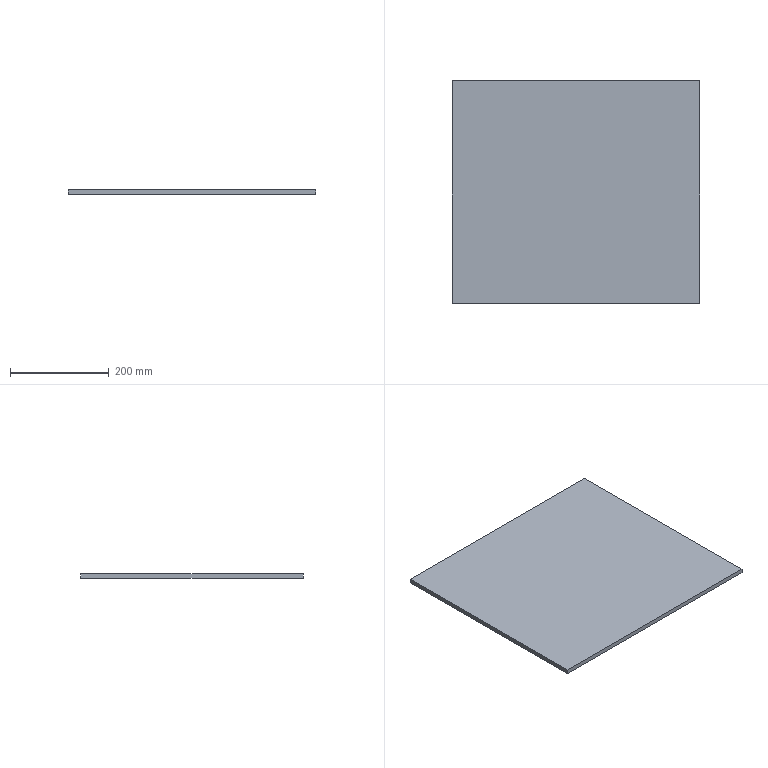Part | NX | 1 solid | 6 faces | box 500 x 450 x 9 mm | volume 2025000 mm3 | plane 6
STEP:
#1=CARTESIAN_POINT('',(-409.726,-361.015,0.));
#2=VERTEX_POINT('',#1);
#3=CARTESIAN_POINT('',(90.274,-361.015,0.));
#4=VERTEX_POINT('',#3);
#5=CARTESIAN_POINT('',(-369.726,-361.015,0.));
#6=DIRECTION('',(1.,0.,0.));
#7=VECTOR('',#6,1000.);
#8=LINE('',#5,#7);
#9=EDGE_CURVE('',#2,#4,#8,.T.);
#10=ORIENTED_EDGE('',*,*,#9,.T.);
#11=CARTESIAN_POINT('',(90.274,-361.015,9.));
#12=VERTEX_POINT('',#11);
#13=CARTESIAN_POINT('',(90.274,-361.015,0.));
#14=DIRECTION('',(0.,0.,1.));
#15=VECTOR('',#14,1000.);
#16=LINE('',#13,#15);
#17=EDGE_CURVE('',#4,#12,#16,.T.);
#18=ORIENTED_EDGE('',*,*,#17,.T.);
#19=CARTESIAN_POINT('',(-409.726,-361.015,9.));
#20=VERTEX_POINT('',#19);
#21=CARTESIAN_POINT('',(-369.726,-361.015,9.));
#22=DIRECTION('',(1.,0.,0.));
#23=VECTOR('',#22,1000.);
#24=LINE('',#21,#23);
#25=EDGE_CURVE('',#20,#12,#24,.T.);
#26=ORIENTED_EDGE('',*,*,#25,.F.);
#27=CARTESIAN_POINT('',(-409.726,-361.015,0.));
#28=DIRECTION('',(0.,0.,1.));
#29=VECTOR('',#28,1000.);
#30=LINE('',#27,#29);
#31=EDGE_CURVE('',#2,#20,#30,.T.);
#32=ORIENTED_EDGE('',*,*,#31,.F.);
#33=EDGE_LOOP('',(#10,#18,#26,#32));
#34=FACE_BOUND('',#33,.T.);
#35=CARTESIAN_POINT('',(90.274,-361.015,0.));
#36=DIRECTION('',(0.,-1.,0.));
#37=DIRECTION('',(0.,0.,-1.));
#38=AXIS2_PLACEMENT_3D('',#35,#36,#37);
#39=PLANE('',#38);
#40=ADVANCED_FACE('',(#34),#39,.T.);
#41=CARTESIAN_POINT('',(90.274,88.985,0.));
#42=VERTEX_POINT('',#41);
#43=CARTESIAN_POINT('',(90.274,48.985,0.));
#44=DIRECTION('',(0.,-1.,0.));
#45=VECTOR('',#44,1000.);
#46=LINE('',#43,#45);
#47=EDGE_CURVE('',#42,#4,#46,.T.);
#48=ORIENTED_EDGE('',*,*,#47,.F.);
#49=CARTESIAN_POINT('',(90.274,88.985,9.));
#50=VERTEX_POINT('',#49);
#51=CARTESIAN_POINT('',(90.274,88.985,0.));
#52=DIRECTION('',(0.,0.,1.));
#53=VECTOR('',#52,1000.);
#54=LINE('',#51,#53);
#55=EDGE_CURVE('',#42,#50,#54,.T.);
#56=ORIENTED_EDGE('',*,*,#55,.T.);
#57=CARTESIAN_POINT('',(90.274,48.985,9.));
#58=DIRECTION('',(0.,-1.,0.));
#59=VECTOR('',#58,1000.);
#60=LINE('',#57,#59);
#61=EDGE_CURVE('',#50,#12,#60,.T.);
#62=ORIENTED_EDGE('',*,*,#61,.T.);
#63=ORIENTED_EDGE('',*,*,#17,.F.);
#64=EDGE_LOOP('',(#48,#56,#62,#63));
#65=FACE_BOUND('',#64,.T.);
#66=CARTESIAN_POINT('',(90.274,88.985,0.));
#67=DIRECTION('',(1.,0.,0.));
#68=DIRECTION('',(0.,1.,0.));
#69=AXIS2_PLACEMENT_3D('',#66,#67,#68);
#70=PLANE('',#69);
#71=ADVANCED_FACE('',(#65),#70,.T.);
#72=CARTESIAN_POINT('',(-409.726,88.985,0.));
#73=VERTEX_POINT('',#72);
#74=CARTESIAN_POINT('',(-369.726,88.985,0.));
#75=DIRECTION('',(1.,0.,0.));
#76=VECTOR('',#75,1000.);
#77=LINE('',#74,#76);
#78=EDGE_CURVE('',#73,#42,#77,.T.);
#79=ORIENTED_EDGE('',*,*,#78,.F.);
#80=CARTESIAN_POINT('',(-409.726,88.985,9.));
#81=VERTEX_POINT('',#80);
#82=CARTESIAN_POINT('',(-409.726,88.985,0.));
#83=DIRECTION('',(0.,0.,1.));
#84=VECTOR('',#83,1000.);
#85=LINE('',#82,#84);
#86=EDGE_CURVE('',#73,#81,#85,.T.);
#87=ORIENTED_EDGE('',*,*,#86,.T.);
#88=CARTESIAN_POINT('',(-369.726,88.985,9.));
#89=DIRECTION('',(1.,0.,0.));
#90=VECTOR('',#89,1000.);
#91=LINE('',#88,#90);
#92=EDGE_CURVE('',#81,#50,#91,.T.);
#93=ORIENTED_EDGE('',*,*,#92,.T.);
#94=ORIENTED_EDGE('',*,*,#55,.F.);
#95=EDGE_LOOP('',(#79,#87,#93,#94));
#96=FACE_BOUND('',#95,.T.);
#97=CARTESIAN_POINT('',(-409.726,88.985,0.));
#98=DIRECTION('',(0.,1.,0.));
#99=DIRECTION('',(1.,0.,0.));
#100=AXIS2_PLACEMENT_3D('',#97,#98,#99);
#101=PLANE('',#100);
#102=ADVANCED_FACE('',(#96),#101,.T.);
#103=CARTESIAN_POINT('',(-409.726,48.985,0.));
#104=DIRECTION('',(0.,-1.,0.));
#105=VECTOR('',#104,1000.);
#106=LINE('',#103,#105);
#107=EDGE_CURVE('',#73,#2,#106,.T.);
#108=ORIENTED_EDGE('',*,*,#107,.T.);
#109=ORIENTED_EDGE('',*,*,#31,.T.);
#110=CARTESIAN_POINT('',(-409.726,48.985,9.));
#111=DIRECTION('',(0.,-1.,0.));
#112=VECTOR('',#111,1000.);
#113=LINE('',#110,#112);
#114=EDGE_CURVE('',#81,#20,#113,.T.);
#115=ORIENTED_EDGE('',*,*,#114,.F.);
#116=ORIENTED_EDGE('',*,*,#86,.F.);
#117=EDGE_LOOP('',(#108,#109,#115,#116));
#118=FACE_BOUND('',#117,.T.);
#119=CARTESIAN_POINT('',(-409.726,-361.015,0.));
#120=DIRECTION('',(-1.,0.,0.));
#121=DIRECTION('',(0.,0.,1.));
#122=AXIS2_PLACEMENT_3D('',#119,#120,#121);
#123=PLANE('',#122);
#124=ADVANCED_FACE('',(#118),#123,.T.);
#125=ORIENTED_EDGE('',*,*,#114,.T.);
#126=ORIENTED_EDGE('',*,*,#25,.T.);
#127=ORIENTED_EDGE('',*,*,#61,.F.);
#128=ORIENTED_EDGE('',*,*,#92,.F.);
#129=EDGE_LOOP('',(#125,#126,#127,#128));
#130=FACE_BOUND('',#129,.T.);
#131=CARTESIAN_POINT('',(-273.242,-346.647,9.));
#132=DIRECTION('',(0.,0.,1.));
#133=DIRECTION('',(1.,0.,0.));
#134=AXIS2_PLACEMENT_3D('',#131,#132,#133);
#135=PLANE('',#134);
#136=ADVANCED_FACE('',(#130),#135,.T.);
#137=ORIENTED_EDGE('',*,*,#78,.T.);
#138=ORIENTED_EDGE('',*,*,#47,.T.);
#139=ORIENTED_EDGE('',*,*,#9,.F.);
#140=ORIENTED_EDGE('',*,*,#107,.F.);
#141=EDGE_LOOP('',(#137,#138,#139,#140));
#142=FACE_BOUND('',#141,.T.);
#143=CARTESIAN_POINT('',(-273.242,-346.647,0.));
#144=DIRECTION('',(0.,0.,1.));
#145=DIRECTION('',(1.,0.,0.));
#146=AXIS2_PLACEMENT_3D('',#143,#144,#145);
#147=PLANE('',#146);
#148=ADVANCED_FACE('',(#142),#147,.F.);
#149=CLOSED_SHELL('',(#40,#71,#102,#124,#136,#148));
#150=MANIFOLD_SOLID_BREP('',#149);
#151=(LENGTH_UNIT()NAMED_UNIT(*)SI_UNIT(.MILLI.,.METRE.));
#152=UNCERTAINTY_MEASURE_WITH_UNIT(LENGTH_MEASURE(0.00001),#151,'','');
#153=(NAMED_UNIT(*)PLANE_ANGLE_UNIT()SI_UNIT($,.RADIAN.));
#154=(NAMED_UNIT(*)SI_UNIT($,.STERADIAN.)SOLID_ANGLE_UNIT());
#155=(GEOMETRIC_REPRESENTATION_CONTEXT(3)GLOBAL_UNCERTAINTY_ASSIGNED_CONTEXT((#152))GLOBAL_UNIT_ASSIGNED_CONTEXT((#151,#153,#154))REPRESENTATION_CONTEXT('',''));
#156=ADVANCED_BREP_SHAPE_REPRESENTATION('',(#150),#155);